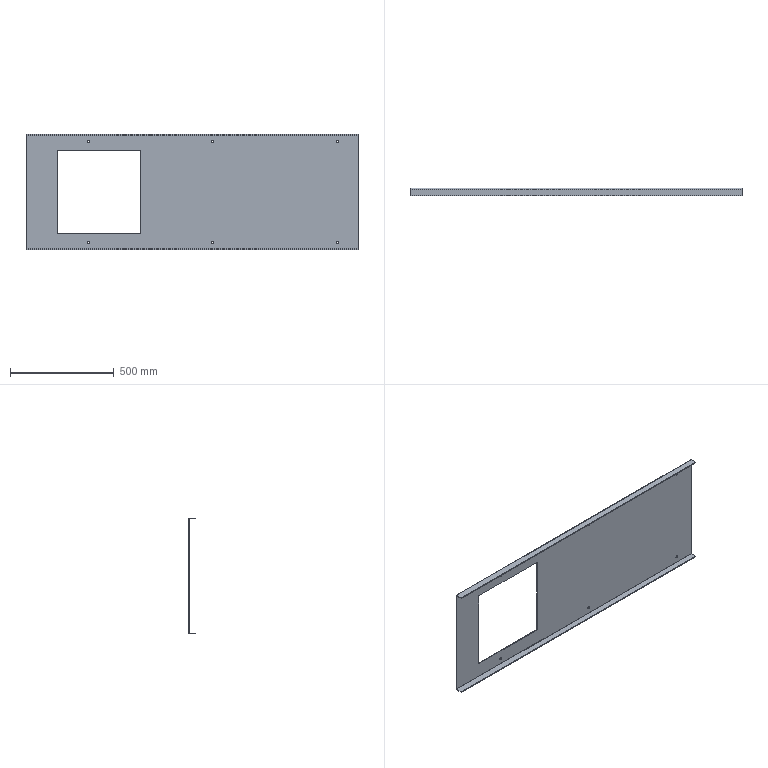Part | STEP file | Input 115 | 1 solid | 30 faces | box 1600 x 35 x 559 mm | volume 3723950 mm3 | cylinder 16 | plane 14 | commonest cylinder face diameters 12 x12 1 x2 10 x2